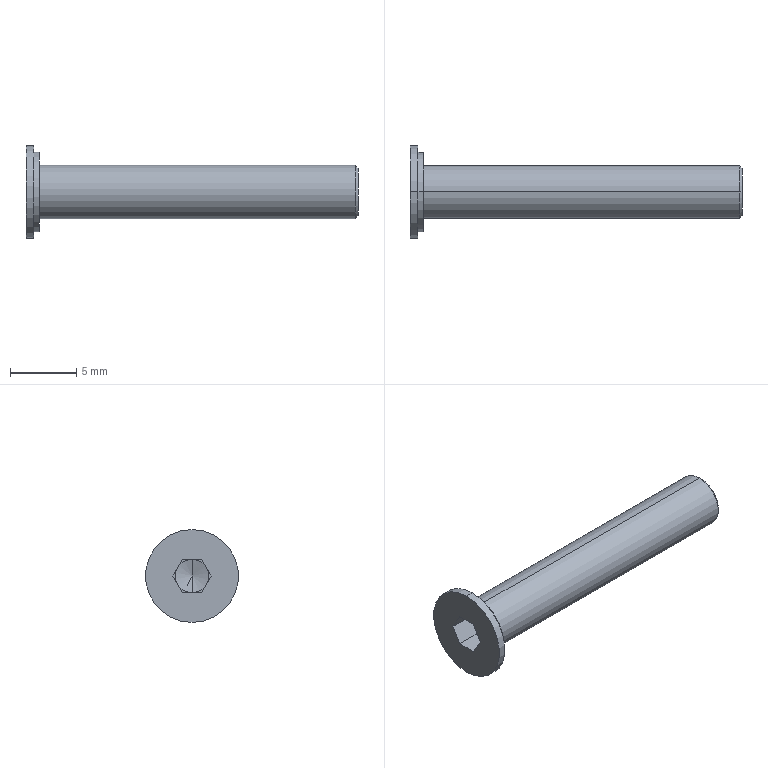Part | STEP file | 11-FG-SZ013 M411_FB4-20 | 1 solid | 26 faces | box 25 x 7 x 7 mm | volume 325.243 mm3 | plane 16 | cylinder 6 | cone 4 | commonest cylinder face diameters 4 x2 6 x2 7 x2